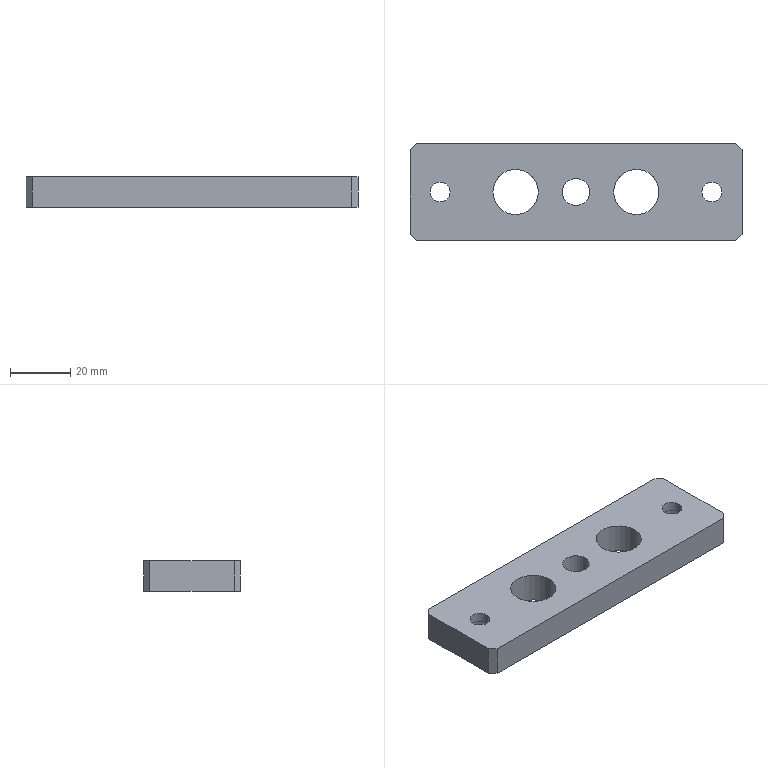Part | STEP file | Probe fixing plate | 1 solid | 26 faces | box 110 x 32 x 10 mm | volume 29438 mm3 | cylinder 14 | plane 12 | commonest cylinder face diameters 6.6 x4 11 x4 15 x4 9 x2